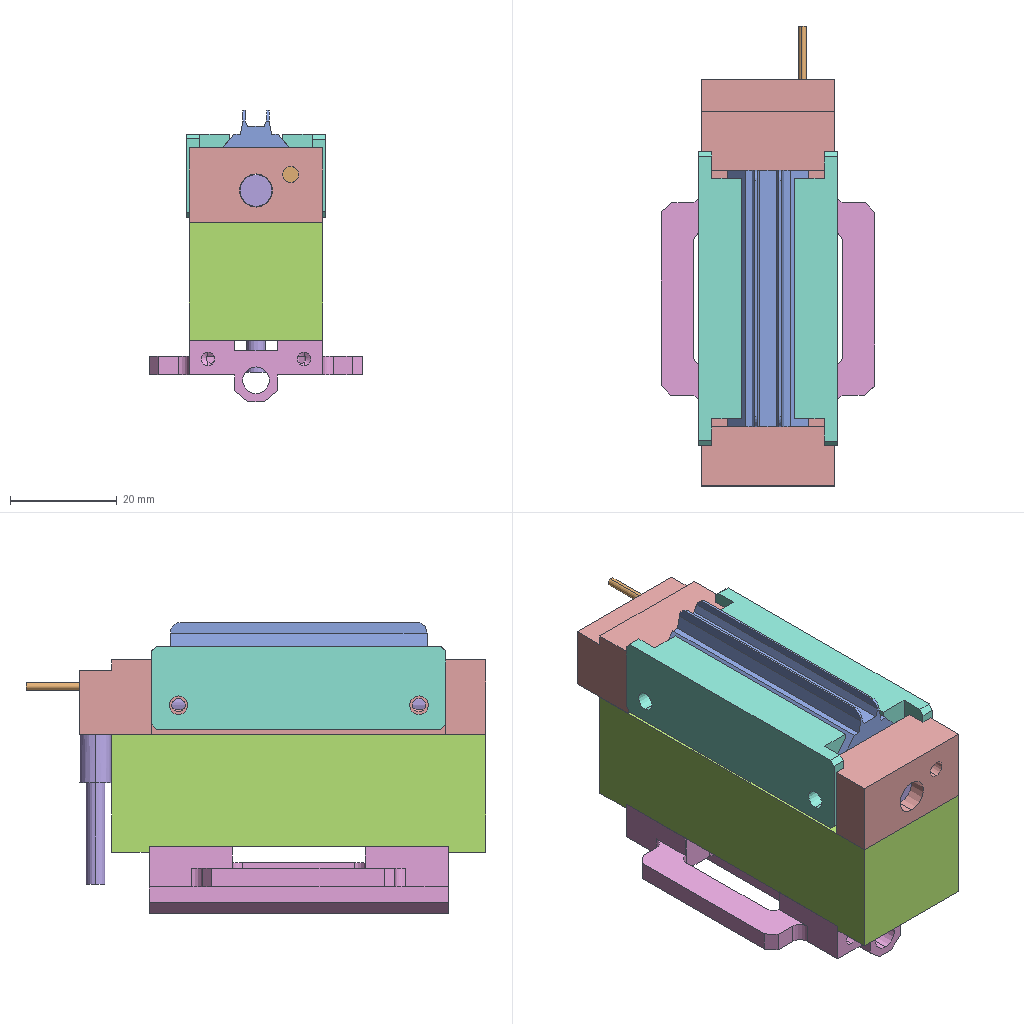Assembly | SolidWorks | 7 different items | 8 placed | box 40 x 86 x 54 mm
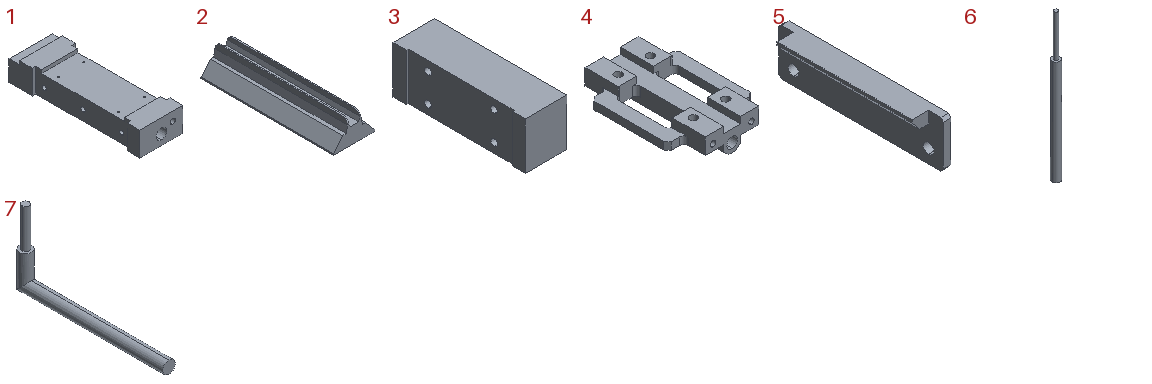Parts list (item | quantity | size | volume | features):
1 | x1 | 25 x 76 x 14 mm | 17689 mm3 | features ICE 7, 3DProfileFeature 4, HoleWzd 4, Extrusion 1, MirrorPattern 1
2 | x1 | 15 x 48 x 9 mm | 3152 mm3 | features Chamfer 6, Extrusion 1, Fillet 1
3 | x1 | 22 x 70 x 25 mm | 36292 mm3 | features ICE 2, Extrusion 1
4 | x1 | 40 x 56 x 12.5 mm | 7758 mm3 | features ICE 7, Chamfer 2, Fillet 2, HoleWzd 2, Extrusion 1
5 | x2 | 8 x 55 x 15.5 mm | 2899 mm3 | features ICE 3, Chamfer 2, Extrusion 1
6 | x1 | 3 x 3 x 56 mm | 311.018 mm3 | features Extrusion 1, ICE 1
7 | x1 | 6 x 73 x 37 mm | 2586 mm3 | features ICE 4, Extrusion 1
Mates (type | each side: item.copy, entity, surface, feature):
Coincident | 2.1 face plane Boss-Extrude1 | 1.1 face plane Boss-Extrude1
DistanceDim | 1.1 face plane Boss-Extrude1 | 2.1 face plane Boss-Extrude1
Coincident | 1.1 face plane Boss-Extrude1 | 3.1 face plane Boss-Extrude1 | 3 times
Concentric | 1.1 face cylinder Cut-Extrude1 | 6.1 face cylinder Boss-Extrude1
Concentric | 1.1 face cylinder Cut-Extrude1 | 7.1 face cylinder Boss-Extrude1
Parallel | 1.1 face plane Boss-Extrude1 | 7.1 face plane Boss-Extrude3
DistanceDim | 1.1 face plane Boss-Extrude1 | 7.1 face plane Boss-Extrude1
Coincident | 1.1 face plane Cut-Extrude3 | 6.1 face plane Boss-Extrude1
Coincident | 1.1 face plane Cut-Extrude4 | 5.1 face plane Cut-Extrude1
Coincident | 1.1 face plane Cut-Extrude4 | 5.2 face plane Cut-Extrude1
Coincident | 1.1 face plane Boss-Extrude2 | 2.1 face plane Boss-Extrude1
Coincident | 3.1 face plane Cut-Extrude3 | 4.1 face plane Boss-Extrude1
Concentric | 1.1 face cylinder M3 Tapped Hole1 | 5.1 face cylinder Cut-Extrude2 | 2 times
Concentric | 1.1 face cylinder Mirror1 | 5.2 face cylinder Cut-Extrude2 | 2 times
Concentric | 3.1 face cylinder Cut-Extrude1 | 4.1 face cylinder Cut-Extrude5 | 2 times